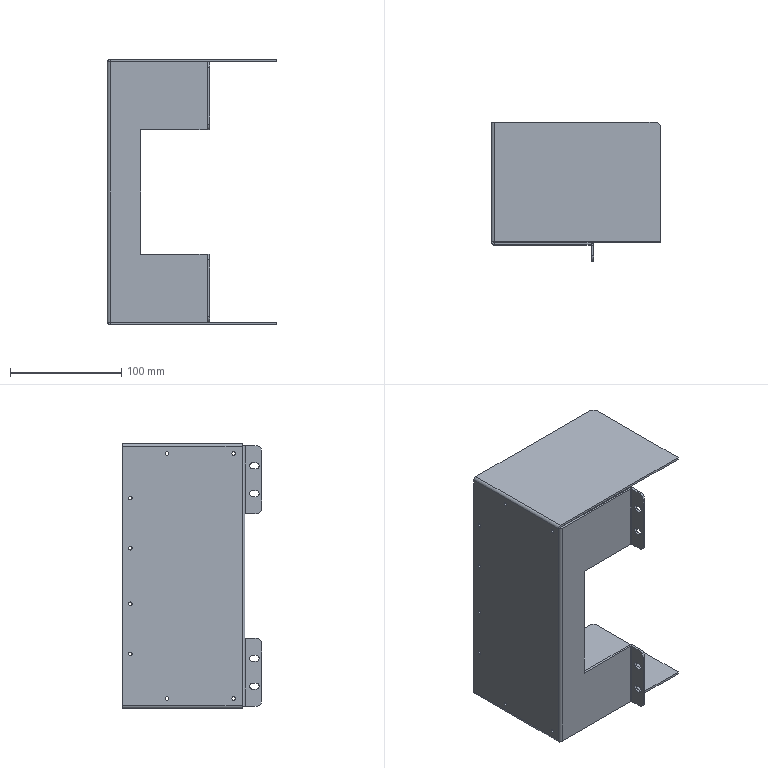Part | STEP file | 1 solid | 90 faces | box 152 x 125 x 238 mm | volume 147473 mm3 | plane 50 | cylinder 40 | commonest cylinder face diameters 3.3 x16 5.5 x8 10 x6 1 x5 5 x5